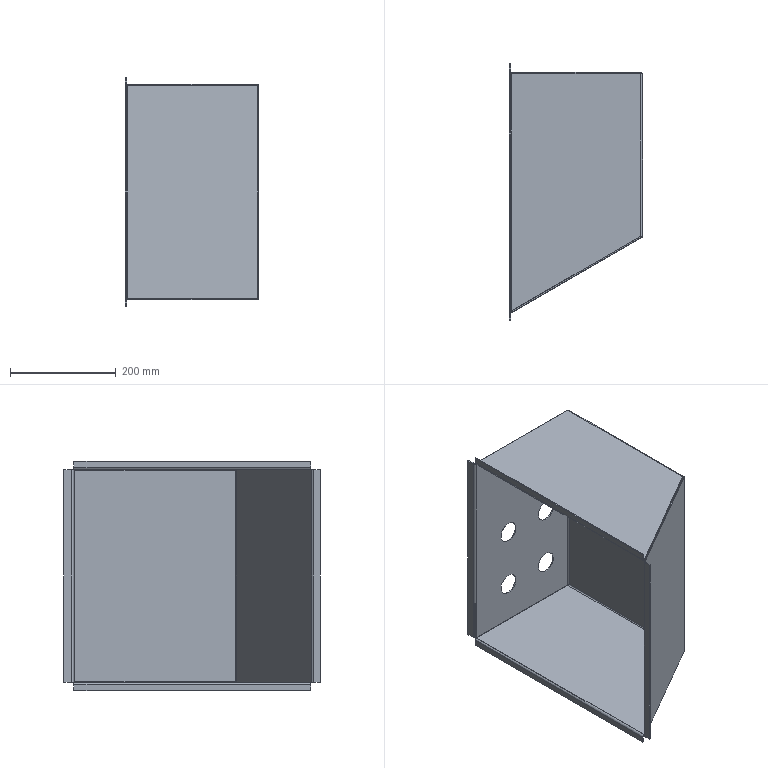Part | STEP file | 750038491 | 1 solid | 68 faces | box 252 x 486 x 434 mm | volume 1098230 mm3 | plane 44 | cylinder 24 | commonest cylinder face diameters 4 x8 8 x8 40 x8